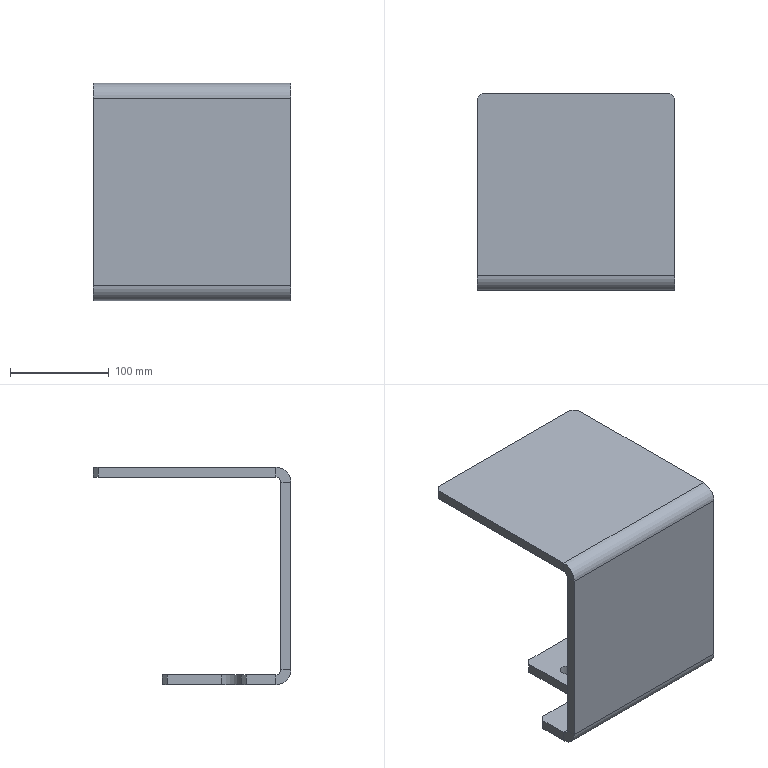Part | SolidWorks | features ICE 4, Fillet 3, Chamfer 1, Extrusion 1, FlatPattern 1, SheetMetal 1, SolidToSheetMetal 1 | 1 solid | 38 faces | box 200 x 200 x 220 mm | volume 944720 mm3 | plane 28 | cylinder 10 | commonest cylinder face diameters 14 x4 10 x2 30 x2 40 x2
STEP:
#1=CARTESIAN_POINT('',(67.,-40.,0.));
#2=VERTEX_POINT('',#1);
#3=CARTESIAN_POINT('',(53.,-40.,0.));
#4=VERTEX_POINT('',#3);
#5=CARTESIAN_POINT('',(60.,-40.,0.));
#6=DIRECTION('',(0.,0.,-1.));
#7=DIRECTION('',(1.,0.,0.));
#8=AXIS2_PLACEMENT_3D('',#5,#6,#7);
#9=CIRCLE('',#8,7.);
#10=EDGE_CURVE('',#2,#4,#9,.T.);
#11=ORIENTED_EDGE('',*,*,#10,.T.);
#12=CARTESIAN_POINT('',(53.,-40.,10.));
#13=VERTEX_POINT('',#12);
#14=CARTESIAN_POINT('',(53.,-40.,10.));
#15=DIRECTION('',(0.,0.,1.));
#16=VECTOR('',#15,1000.);
#17=LINE('',#14,#16);
#18=EDGE_CURVE('',#4,#13,#17,.T.);
#19=ORIENTED_EDGE('',*,*,#18,.T.);
#20=CARTESIAN_POINT('',(67.,-40.,10.));
#21=VERTEX_POINT('',#20);
#22=CARTESIAN_POINT('',(60.,-40.,10.));
#23=DIRECTION('',(0.,0.,-1.));
#24=DIRECTION('',(1.,0.,0.));
#25=AXIS2_PLACEMENT_3D('',#22,#23,#24);
#26=CIRCLE('',#25,7.);
#27=EDGE_CURVE('',#21,#13,#26,.T.);
#28=ORIENTED_EDGE('',*,*,#27,.F.);
#29=CARTESIAN_POINT('',(67.,-40.,10.));
#30=DIRECTION('',(0.,0.,1.));
#31=VECTOR('',#30,1000.);
#32=LINE('',#29,#31);
#33=EDGE_CURVE('',#2,#21,#32,.T.);
#34=ORIENTED_EDGE('',*,*,#33,.F.);
#35=EDGE_LOOP('',(#11,#19,#28,#34));
#36=FACE_OUTER_BOUND('',#35,.T.);
#37=CARTESIAN_POINT('',(60.,-40.,10.));
#38=DIRECTION('',(0.,0.,1.));
#39=DIRECTION('',(1.,0.,0.));
#40=AXIS2_PLACEMENT_3D('',#37,#38,#39);
#41=CYLINDRICAL_SURFACE('',#40,7.);
#42=ADVANCED_FACE('',(#36),#41,.F.);
#43=CARTESIAN_POINT('',(27.,-40.,0.));
#44=VERTEX_POINT('',#43);
#45=CARTESIAN_POINT('',(13.,-40.,0.));
#46=VERTEX_POINT('',#45);
#47=CARTESIAN_POINT('',(20.,-40.,0.));
#48=DIRECTION('',(0.,0.,-1.));
#49=DIRECTION('',(1.,0.,0.));
#50=AXIS2_PLACEMENT_3D('',#47,#48,#49);
#51=CIRCLE('',#50,7.);
#52=EDGE_CURVE('',#44,#46,#51,.T.);
#53=ORIENTED_EDGE('',*,*,#52,.T.);
#54=CARTESIAN_POINT('',(13.,-40.,10.));
#55=VERTEX_POINT('',#54);
#56=CARTESIAN_POINT('',(13.,-40.,10.));
#57=DIRECTION('',(0.,0.,1.));
#58=VECTOR('',#57,1000.);
#59=LINE('',#56,#58);
#60=EDGE_CURVE('',#46,#55,#59,.T.);
#61=ORIENTED_EDGE('',*,*,#60,.T.);
#62=CARTESIAN_POINT('',(27.,-40.,10.));
#63=VERTEX_POINT('',#62);
#64=CARTESIAN_POINT('',(20.,-40.,10.));
#65=DIRECTION('',(0.,0.,-1.));
#66=DIRECTION('',(1.,0.,0.));
#67=AXIS2_PLACEMENT_3D('',#64,#65,#66);
#68=CIRCLE('',#67,7.);
#69=EDGE_CURVE('',#63,#55,#68,.T.);
#70=ORIENTED_EDGE('',*,*,#69,.F.);
#71=CARTESIAN_POINT('',(27.,-40.,10.));
#72=DIRECTION('',(0.,0.,1.));
#73=VECTOR('',#72,1000.);
#74=LINE('',#71,#73);
#75=EDGE_CURVE('',#44,#63,#74,.T.);
#76=ORIENTED_EDGE('',*,*,#75,.F.);
#77=EDGE_LOOP('',(#53,#61,#70,#76));
#78=FACE_OUTER_BOUND('',#77,.T.);
#79=CARTESIAN_POINT('',(20.,-40.,10.));
#80=DIRECTION('',(0.,0.,1.));
#81=DIRECTION('',(1.,0.,0.));
#82=AXIS2_PLACEMENT_3D('',#79,#80,#81);
#83=CYLINDRICAL_SURFACE('',#82,7.);
#84=ADVANCED_FACE('',(#78),#83,.F.);
#85=CARTESIAN_POINT('',(140.,-130.,15.));
#86=VERTEX_POINT('',#85);
#87=CARTESIAN_POINT('',(140.,-120.,15.));
#88=VERTEX_POINT('',#87);
#89=CARTESIAN_POINT('',(140.,-120.,15.));
#90=DIRECTION('',(0.,1.,0.));
#91=VECTOR('',#90,1000.);
#92=LINE('',#89,#91);
#93=EDGE_CURVE('',#86,#88,#92,.T.);
#94=ORIENTED_EDGE('',*,*,#93,.F.);
#95=CARTESIAN_POINT('',(140.,-115.,0.));
#96=VERTEX_POINT('',#95);
#97=CARTESIAN_POINT('',(140.,-115.,15.));
#98=DIRECTION('',(-1.,0.,0.));
#99=DIRECTION('',(0.,0.,1.));
#100=AXIS2_PLACEMENT_3D('',#97,#98,#99);
#101=CIRCLE('',#100,15.);
#102=EDGE_CURVE('',#96,#86,#101,.T.);
#103=ORIENTED_EDGE('',*,*,#102,.F.);
#104=CARTESIAN_POINT('',(140.,-115.,10.));
#105=VERTEX_POINT('',#104);
#106=CARTESIAN_POINT('',(140.,-115.,10.));
#107=DIRECTION('',(0.,0.,1.));
#108=VECTOR('',#107,1000.);
#109=LINE('',#106,#108);
#110=EDGE_CURVE('',#96,#105,#109,.T.);
#111=ORIENTED_EDGE('',*,*,#110,.T.);
#112=CARTESIAN_POINT('',(140.,-115.,15.));
#113=DIRECTION('',(-1.,0.,0.));
#114=DIRECTION('',(0.,1.,0.));
#115=AXIS2_PLACEMENT_3D('',#112,#113,#114);
#116=CIRCLE('',#115,5.);
#117=EDGE_CURVE('',#105,#88,#116,.T.);
#118=ORIENTED_EDGE('',*,*,#117,.T.);
#119=EDGE_LOOP('',(#94,#103,#111,#118));
#120=FACE_OUTER_BOUND('',#119,.T.);
#121=CARTESIAN_POINT('',(140.,-115.,15.));
#122=DIRECTION('',(-1.,0.,0.));
#123=DIRECTION('',(0.,-1.,0.));
#124=AXIS2_PLACEMENT_3D('',#121,#122,#123);
#125=PLANE('',#124);
#126=ADVANCED_FACE('',(#120),#125,.F.);
#127=ORIENTED_EDGE('',*,*,#110,.F.);
#128=CARTESIAN_POINT('',(140.,-85.,0.));
#129=VERTEX_POINT('',#128);
#130=CARTESIAN_POINT('',(140.,0.,0.));
#131=DIRECTION('',(0.,1.,0.));
#132=VECTOR('',#131,1000.);
#133=LINE('',#130,#132);
#134=EDGE_CURVE('',#96,#129,#133,.T.);
#135=ORIENTED_EDGE('',*,*,#134,.T.);
#136=CARTESIAN_POINT('',(140.,-85.,10.));
#137=VERTEX_POINT('',#136);
#138=CARTESIAN_POINT('',(140.,-85.,10.));
#139=DIRECTION('',(0.,0.,1.));
#140=VECTOR('',#139,1000.);
#141=LINE('',#138,#140);
#142=EDGE_CURVE('',#129,#137,#141,.T.);
#143=ORIENTED_EDGE('',*,*,#142,.T.);
#144=CARTESIAN_POINT('',(140.,-80.,10.));
#145=DIRECTION('',(0.,1.,0.));
#146=VECTOR('',#145,1000.);
#147=LINE('',#144,#146);
#148=EDGE_CURVE('',#105,#137,#147,.T.);
#149=ORIENTED_EDGE('',*,*,#148,.F.);
#150=EDGE_LOOP('',(#127,#135,#143,#149));
#151=FACE_OUTER_BOUND('',#150,.T.);
#152=CARTESIAN_POINT('',(140.,-80.,10.));
#153=DIRECTION('',(1.,0.,0.));
#154=DIRECTION('',(0.,1.,0.));
#155=AXIS2_PLACEMENT_3D('',#152,#153,#154);
#156=PLANE('',#155);
#157=ADVANCED_FACE('',(#151),#156,.T.);
#158=ORIENTED_EDGE('',*,*,#142,.F.);
#159=CARTESIAN_POINT('',(135.,-80.,0.));
#160=VERTEX_POINT('',#159);
#161=CARTESIAN_POINT('',(27.5,27.5,0.));
#162=DIRECTION('',(-0.7071,0.7071,0.));
#163=VECTOR('',#162,1000.);
#164=LINE('',#161,#163);
#165=EDGE_CURVE('',#129,#160,#164,.T.);
#166=ORIENTED_EDGE('',*,*,#165,.T.);
#167=CARTESIAN_POINT('',(135.,-80.,10.));
#168=VERTEX_POINT('',#167);
#169=CARTESIAN_POINT('',(135.,-80.,10.));
#170=DIRECTION('',(0.,0.,1.));
#171=VECTOR('',#170,1000.);
#172=LINE('',#169,#171);
#173=EDGE_CURVE('',#160,#168,#172,.T.);
#174=ORIENTED_EDGE('',*,*,#173,.T.);
#175=CARTESIAN_POINT('',(27.5,27.5,10.));
#176=DIRECTION('',(-0.7071,0.7071,0.));
#177=VECTOR('',#176,1000.);
#178=LINE('',#175,#177);
#179=EDGE_CURVE('',#137,#168,#178,.T.);
#180=ORIENTED_EDGE('',*,*,#179,.F.);
#181=EDGE_LOOP('',(#158,#166,#174,#180));
#182=FACE_OUTER_BOUND('',#181,.T.);
#183=CARTESIAN_POINT('',(27.5,27.5,10.));
#184=DIRECTION('',(-0.7071,-0.7071,0.));
#185=DIRECTION('',(0.7071,-0.7071,0.));
#186=AXIS2_PLACEMENT_3D('',#183,#184,#185);
#187=PLANE('',#186);
#188=ADVANCED_FACE('',(#182),#187,.F.);
#189=ORIENTED_EDGE('',*,*,#173,.F.);
#190=CARTESIAN_POINT('',(100.,-80.,0.));
#191=VERTEX_POINT('',#190);
#192=CARTESIAN_POINT('',(0.,-80.,0.));
#193=DIRECTION('',(-1.,0.,0.));
#194=VECTOR('',#193,1000.);
#195=LINE('',#192,#194);
#196=EDGE_CURVE('',#160,#191,#195,.T.);
#197=ORIENTED_EDGE('',*,*,#196,.T.);
#198=CARTESIAN_POINT('',(100.,-80.,10.));
#199=VERTEX_POINT('',#198);
#200=CARTESIAN_POINT('',(100.,-80.,10.));
#201=DIRECTION('',(0.,0.,1.));
#202=VECTOR('',#201,1000.);
#203=LINE('',#200,#202);
#204=EDGE_CURVE('',#191,#199,#203,.T.);
#205=ORIENTED_EDGE('',*,*,#204,.T.);
#206=CARTESIAN_POINT('',(-60.,-80.,10.));
#207=DIRECTION('',(-1.,0.,0.));
#208=VECTOR('',#207,1000.);
#209=LINE('',#206,#208);
#210=EDGE_CURVE('',#168,#199,#209,.T.);
#211=ORIENTED_EDGE('',*,*,#210,.F.);
#212=EDGE_LOOP('',(#189,#197,#205,#211));
#213=FACE_OUTER_BOUND('',#212,.T.);
#214=CARTESIAN_POINT('',(-60.,-80.,10.));
#215=DIRECTION('',(0.,1.,0.));
#216=DIRECTION('',(-1.,0.,0.));
#217=AXIS2_PLACEMENT_3D('',#214,#215,#216);
#218=PLANE('',#217);
#219=ADVANCED_FACE('',(#213),#218,.T.);
#220=ORIENTED_EDGE('',*,*,#204,.F.);
#221=CARTESIAN_POINT('',(80.,-60.,0.));
#222=VERTEX_POINT('',#221);
#223=CARTESIAN_POINT('',(100.,-60.,0.));
#224=DIRECTION('',(0.,0.,-1.));
#225=DIRECTION('',(1.,0.,0.));
#226=AXIS2_PLACEMENT_3D('',#223,#224,#225);
#227=CIRCLE('',#226,20.);
#228=EDGE_CURVE('',#191,#222,#227,.T.);
#229=ORIENTED_EDGE('',*,*,#228,.T.);
#230=CARTESIAN_POINT('',(80.,-60.,10.));
#231=VERTEX_POINT('',#230);
#232=CARTESIAN_POINT('',(80.,-60.,10.));
#233=DIRECTION('',(0.,0.,1.));
#234=VECTOR('',#233,1000.);
#235=LINE('',#232,#234);
#236=EDGE_CURVE('',#222,#231,#235,.T.);
#237=ORIENTED_EDGE('',*,*,#236,.T.);
#238=CARTESIAN_POINT('',(100.,-60.,10.));
#239=DIRECTION('',(0.,0.,-1.));
#240=DIRECTION('',(1.,0.,0.));
#241=AXIS2_PLACEMENT_3D('',#238,#239,#240);
#242=CIRCLE('',#241,20.);
#243=EDGE_CURVE('',#199,#231,#242,.T.);
#244=ORIENTED_EDGE('',*,*,#243,.F.);
#245=EDGE_LOOP('',(#220,#229,#237,#244));
#246=FACE_OUTER_BOUND('',#245,.T.);
#247=CARTESIAN_POINT('',(100.,-60.,10.));
#248=DIRECTION('',(0.,0.,1.));
#249=DIRECTION('',(1.,0.,0.));
#250=AXIS2_PLACEMENT_3D('',#247,#248,#249);
#251=CYLINDRICAL_SURFACE('',#250,20.);
#252=ADVANCED_FACE('',(#246),#251,.F.);
#253=ORIENTED_EDGE('',*,*,#236,.F.);
#254=CARTESIAN_POINT('',(80.,-5.,0.));
#255=VERTEX_POINT('',#254);
#256=CARTESIAN_POINT('',(80.,0.,0.));
#257=DIRECTION('',(0.,1.,0.));
#258=VECTOR('',#257,1000.);
#259=LINE('',#256,#258);
#260=EDGE_CURVE('',#222,#255,#259,.T.);
#261=ORIENTED_EDGE('',*,*,#260,.T.);
#262=CARTESIAN_POINT('',(80.,-5.,10.));
#263=VERTEX_POINT('',#262);
#264=CARTESIAN_POINT('',(80.,-5.,10.));
#265=DIRECTION('',(0.,0.,1.));
#266=VECTOR('',#265,1000.);
#267=LINE('',#264,#266);
#268=EDGE_CURVE('',#255,#263,#267,.T.);
#269=ORIENTED_EDGE('',*,*,#268,.T.);
#270=CARTESIAN_POINT('',(80.,0.,10.));
#271=DIRECTION('',(0.,1.,0.));
#272=VECTOR('',#271,1000.);
#273=LINE('',#270,#272);
#274=EDGE_CURVE('',#231,#263,#273,.T.);
#275=ORIENTED_EDGE('',*,*,#274,.F.);
#276=EDGE_LOOP('',(#253,#261,#269,#275));
#277=FACE_OUTER_BOUND('',#276,.T.);
#278=CARTESIAN_POINT('',(80.,0.,10.));
#279=DIRECTION('',(1.,0.,0.));
#280=DIRECTION('',(0.,1.,0.));
#281=AXIS2_PLACEMENT_3D('',#278,#279,#280);
#282=PLANE('',#281);
#283=ADVANCED_FACE('',(#277),#282,.T.);
#284=ORIENTED_EDGE('',*,*,#268,.F.);
#285=CARTESIAN_POINT('',(75.,0.,0.));
#286=VERTEX_POINT('',#285);
#287=CARTESIAN_POINT('',(37.5,37.5,0.));
#288=DIRECTION('',(-0.7071,0.7071,0.));
#289=VECTOR('',#288,1000.);
#290=LINE('',#287,#289);
#291=EDGE_CURVE('',#255,#286,#290,.T.);
#292=ORIENTED_EDGE('',*,*,#291,.T.);
#293=CARTESIAN_POINT('',(75.,0.,10.));
#294=VERTEX_POINT('',#293);
#295=CARTESIAN_POINT('',(75.,0.,10.));
#296=DIRECTION('',(0.,0.,1.));
#297=VECTOR('',#296,1000.);
#298=LINE('',#295,#297);
#299=EDGE_CURVE('',#286,#294,#298,.T.);
#300=ORIENTED_EDGE('',*,*,#299,.T.);
#301=CARTESIAN_POINT('',(37.5,37.5,10.));
#302=DIRECTION('',(-0.7071,0.7071,0.));
#303=VECTOR('',#302,1000.);
#304=LINE('',#301,#303);
#305=EDGE_CURVE('',#263,#294,#304,.T.);
#306=ORIENTED_EDGE('',*,*,#305,.F.);
#307=EDGE_LOOP('',(#284,#292,#300,#306));
#308=FACE_OUTER_BOUND('',#307,.T.);
#309=CARTESIAN_POINT('',(37.5,37.5,10.));
#310=DIRECTION('',(-0.7071,-0.7071,0.));
#311=DIRECTION('',(0.7071,-0.7071,0.));
#312=AXIS2_PLACEMENT_3D('',#309,#310,#311);
#313=PLANE('',#312);
#314=ADVANCED_FACE('',(#308),#313,.F.);
#315=ORIENTED_EDGE('',*,*,#299,.F.);
#316=CARTESIAN_POINT('',(5.,0.,0.));
#317=VERTEX_POINT('',#316);
#318=CARTESIAN_POINT('',(0.,0.,0.));
#319=DIRECTION('',(-1.,0.,0.));
#320=VECTOR('',#319,1000.);
#321=LINE('',#318,#320);
#322=EDGE_CURVE('',#286,#317,#321,.T.);
#323=ORIENTED_EDGE('',*,*,#322,.T.);
#324=CARTESIAN_POINT('',(5.,0.,10.));
#325=VERTEX_POINT('',#324);
#326=CARTESIAN_POINT('',(5.,0.,10.));
#327=DIRECTION('',(0.,0.,1.));
#328=VECTOR('',#327,1000.);
#329=LINE('',#326,#328);
#330=EDGE_CURVE('',#317,#325,#329,.T.);
#331=ORIENTED_EDGE('',*,*,#330,.T.);
#332=CARTESIAN_POINT('',(0.,0.,10.));
#333=DIRECTION('',(-1.,0.,0.));
#334=VECTOR('',#333,1000.);
#335=LINE('',#332,#334);
#336=EDGE_CURVE('',#294,#325,#335,.T.);
#337=ORIENTED_EDGE('',*,*,#336,.F.);
#338=EDGE_LOOP('',(#315,#323,#331,#337));
#339=FACE_OUTER_BOUND('',#338,.T.);
#340=CARTESIAN_POINT('',(0.,0.,10.));
#341=DIRECTION('',(0.,1.,0.));
#342=DIRECTION('',(-1.,0.,0.));
#343=AXIS2_PLACEMENT_3D('',#340,#341,#342);
#344=PLANE('',#343);
#345=ADVANCED_FACE('',(#339),#344,.T.);
#346=ORIENTED_EDGE('',*,*,#330,.F.);
#347=CARTESIAN_POINT('',(0.,-5.,0.));
#348=VERTEX_POINT('',#347);
#349=CARTESIAN_POINT('',(2.5,-2.5,0.));
#350=DIRECTION('',(-0.7071,-0.7071,0.));
#351=VECTOR('',#350,1000.);
#352=LINE('',#349,#351);
#353=EDGE_CURVE('',#317,#348,#352,.T.);
#354=ORIENTED_EDGE('',*,*,#353,.T.);
#355=CARTESIAN_POINT('',(0.,-5.,10.));
#356=VERTEX_POINT('',#355);
#357=CARTESIAN_POINT('',(0.,-5.,10.));
#358=DIRECTION('',(0.,0.,1.));
#359=VECTOR('',#358,1000.);
#360=LINE('',#357,#359);
#361=EDGE_CURVE('',#348,#356,#360,.T.);
#362=ORIENTED_EDGE('',*,*,#361,.T.);
#363=CARTESIAN_POINT('',(2.5,-2.5,10.));
#364=DIRECTION('',(-0.7071,-0.7071,0.));
#365=VECTOR('',#364,1000.);
#366=LINE('',#363,#365);
#367=EDGE_CURVE('',#325,#356,#366,.T.);
#368=ORIENTED_EDGE('',*,*,#367,.F.);
#369=EDGE_LOOP('',(#346,#354,#362,#368));
#370=FACE_OUTER_BOUND('',#369,.T.);
#371=CARTESIAN_POINT('',(2.5,-2.5,10.));
#372=DIRECTION('',(0.7071,-0.7071,0.));
#373=DIRECTION('',(0.7071,0.7071,0.));
#374=AXIS2_PLACEMENT_3D('',#371,#372,#373);
#375=PLANE('',#374);
#376=ADVANCED_FACE('',(#370),#375,.F.);
#377=ORIENTED_EDGE('',*,*,#361,.F.);
#378=CARTESIAN_POINT('',(0.,-60.,0.));
#379=VERTEX_POINT('',#378);
#380=CARTESIAN_POINT('',(0.,0.,0.));
#381=DIRECTION('',(0.,-1.,0.));
#382=VECTOR('',#381,1000.);
#383=LINE('',#380,#382);
#384=EDGE_CURVE('',#348,#379,#383,.T.);
#385=ORIENTED_EDGE('',*,*,#384,.T.);
#386=CARTESIAN_POINT('',(0.,-60.,10.));
#387=VERTEX_POINT('',#386);
#388=CARTESIAN_POINT('',(0.,-60.,10.));
#389=DIRECTION('',(0.,0.,1.));
#390=VECTOR('',#389,1000.);
#391=LINE('',#388,#390);
#392=EDGE_CURVE('',#379,#387,#391,.T.);
#393=ORIENTED_EDGE('',*,*,#392,.T.);
#394=CARTESIAN_POINT('',(0.,0.,10.));
#395=DIRECTION('',(0.,-1.,0.));
#396=VECTOR('',#395,1000.);
#397=LINE('',#394,#396);
#398=EDGE_CURVE('',#356,#387,#397,.T.);
#399=ORIENTED_EDGE('',*,*,#398,.F.);
#400=EDGE_LOOP('',(#377,#385,#393,#399));
#401=FACE_OUTER_BOUND('',#400,.T.);
#402=CARTESIAN_POINT('',(0.,0.,10.));
#403=DIRECTION('',(-1.,0.,0.));
#404=DIRECTION('',(0.,-1.,0.));
#405=AXIS2_PLACEMENT_3D('',#402,#403,#404);
#406=PLANE('',#405);
#407=ADVANCED_FACE('',(#401),#406,.T.);
#408=ORIENTED_EDGE('',*,*,#392,.F.);
#409=CARTESIAN_POINT('',(-20.,-80.,0.));
#410=VERTEX_POINT('',#409);
#411=CARTESIAN_POINT('',(-20.,-60.,0.));
#412=DIRECTION('',(0.,0.,-1.));
#413=DIRECTION('',(1.,0.,0.));
#414=AXIS2_PLACEMENT_3D('',#411,#412,#413);
#415=CIRCLE('',#414,20.);
#416=EDGE_CURVE('',#379,#410,#415,.T.);
#417=ORIENTED_EDGE('',*,*,#416,.T.);
#418=CARTESIAN_POINT('',(-20.,-80.,10.));
#419=VERTEX_POINT('',#418);
#420=CARTESIAN_POINT('',(-20.,-80.,10.));
#421=DIRECTION('',(0.,0.,1.));
#422=VECTOR('',#421,1000.);
#423=LINE('',#420,#422);
#424=EDGE_CURVE('',#410,#419,#423,.T.);
#425=ORIENTED_EDGE('',*,*,#424,.T.);
#426=CARTESIAN_POINT('',(-20.,-60.,10.));
#427=DIRECTION('',(0.,0.,-1.));
#428=DIRECTION('',(1.,0.,0.));
#429=AXIS2_PLACEMENT_3D('',#426,#427,#428);
#430=CIRCLE('',#429,20.);
#431=EDGE_CURVE('',#387,#419,#430,.T.);
#432=ORIENTED_EDGE('',*,*,#431,.F.);
#433=EDGE_LOOP('',(#408,#417,#425,#432));
#434=FACE_OUTER_BOUND('',#433,.T.);
#435=CARTESIAN_POINT('',(-20.,-60.,10.));
#436=DIRECTION('',(0.,0.,1.));
#437=DIRECTION('',(1.,0.,0.));
#438=AXIS2_PLACEMENT_3D('',#435,#436,#437);
#439=CYLINDRICAL_SURFACE('',#438,20.);
#440=ADVANCED_FACE('',(#434),#439,.F.);
#441=ORIENTED_EDGE('',*,*,#424,.F.);
#442=CARTESIAN_POINT('',(-55.,-80.,0.));
#443=VERTEX_POINT('',#442);
#444=CARTESIAN_POINT('',(0.,-80.,0.));
#445=DIRECTION('',(-1.,0.,0.));
#446=VECTOR('',#445,1000.);
#447=LINE('',#444,#446);
#448=EDGE_CURVE('',#410,#443,#447,.T.);
#449=ORIENTED_EDGE('',*,*,#448,.T.);
#450=CARTESIAN_POINT('',(-55.,-80.,10.));
#451=VERTEX_POINT('',#450);
#452=CARTESIAN_POINT('',(-55.,-80.,10.));
#453=DIRECTION('',(0.,0.,1.));
#454=VECTOR('',#453,1000.);
#455=LINE('',#452,#454);
#456=EDGE_CURVE('',#443,#451,#455,.T.);
#457=ORIENTED_EDGE('',*,*,#456,.T.);
#458=CARTESIAN_POINT('',(-60.,-80.,10.));
#459=DIRECTION('',(-1.,0.,0.));
#460=VECTOR('',#459,1000.);
#461=LINE('',#458,#460);
#462=EDGE_CURVE('',#419,#451,#461,.T.);
#463=ORIENTED_EDGE('',*,*,#462,.F.);
#464=EDGE_LOOP('',(#441,#449,#457,#463));
#465=FACE_OUTER_BOUND('',#464,.T.);
#466=CARTESIAN_POINT('',(-60.,-80.,10.));
#467=DIRECTION('',(0.,1.,0.));
#468=DIRECTION('',(-1.,0.,0.));
#469=AXIS2_PLACEMENT_3D('',#466,#467,#468);
#470=PLANE('',#469);
#471=ADVANCED_FACE('',(#465),#470,.T.);
#472=ORIENTED_EDGE('',*,*,#456,.F.);
#473=CARTESIAN_POINT('',(-60.,-85.,0.));
#474=VERTEX_POINT('',#473);
#475=CARTESIAN_POINT('',(12.5,-12.5,0.));
#476=DIRECTION('',(-0.7071,-0.7071,0.));
#477=VECTOR('',#476,1000.);
#478=LINE('',#475,#477);
#479=EDGE_CURVE('',#443,#474,#478,.T.);
#480=ORIENTED_EDGE('',*,*,#479,.T.);
#481=CARTESIAN_POINT('',(-60.,-85.,10.));
#482=VERTEX_POINT('',#481);
#483=CARTESIAN_POINT('',(-60.,-85.,10.));
#484=DIRECTION('',(0.,0.,1.));
#485=VECTOR('',#484,1000.);
#486=LINE('',#483,#485);
#487=EDGE_CURVE('',#474,#482,#486,.T.);
#488=ORIENTED_EDGE('',*,*,#487,.T.);
#489=CARTESIAN_POINT('',(12.5,-12.5,10.));
#490=DIRECTION('',(-0.7071,-0.7071,0.));
#491=VECTOR('',#490,1000.);
#492=LINE('',#489,#491);
#493=EDGE_CURVE('',#451,#482,#492,.T.);
#494=ORIENTED_EDGE('',*,*,#493,.F.);
#495=EDGE_LOOP('',(#472,#480,#488,#494));
#496=FACE_OUTER_BOUND('',#495,.T.);
#497=CARTESIAN_POINT('',(12.5,-12.5,10.));
#498=DIRECTION('',(0.7071,-0.7071,0.));
#499=DIRECTION('',(0.7071,0.7071,0.));
#500=AXIS2_PLACEMENT_3D('',#497,#498,#499);
#501=PLANE('',#500);
#502=ADVANCED_FACE('',(#496),#501,.F.);
#503=ORIENTED_EDGE('',*,*,#487,.F.);
#504=CARTESIAN_POINT('',(-60.,-115.,0.));
#505=VERTEX_POINT('',#504);
#506=CARTESIAN_POINT('',(-60.,0.,0.));
#507=DIRECTION('',(0.,-1.,0.));
#508=VECTOR('',#507,1000.);
#509=LINE('',#506,#508);
#510=EDGE_CURVE('',#474,#505,#509,.T.);
#511=ORIENTED_EDGE('',*,*,#510,.T.);
#512=CARTESIAN_POINT('',(-60.,-115.,10.));
#513=VERTEX_POINT('',#512);
#514=CARTESIAN_POINT('',(-60.,-115.,10.));
#515=DIRECTION('',(0.,0.,1.));
#516=VECTOR('',#515,1000.);
#517=LINE('',#514,#516);
#518=EDGE_CURVE('',#505,#513,#517,.T.);
#519=ORIENTED_EDGE('',*,*,#518,.T.);
#520=CARTESIAN_POINT('',(-60.,-80.,10.));
#521=DIRECTION('',(0.,-1.,0.));
#522=VECTOR('',#521,1000.);
#523=LINE('',#520,#522);
#524=EDGE_CURVE('',#482,#513,#523,.T.);
#525=ORIENTED_EDGE('',*,*,#524,.F.);
#526=EDGE_LOOP('',(#503,#511,#519,#525));
#527=FACE_OUTER_BOUND('',#526,.T.);
#528=CARTESIAN_POINT('',(-60.,-80.,10.));
#529=DIRECTION('',(-1.,0.,0.));
#530=DIRECTION('',(0.,-1.,0.));
#531=AXIS2_PLACEMENT_3D('',#528,#529,#530);
#532=PLANE('',#531);
#533=ADVANCED_FACE('',(#527),#532,.T.);
#534=ORIENTED_EDGE('',*,*,#518,.F.);
#535=CARTESIAN_POINT('',(-60.,-130.,15.));
#536=VERTEX_POINT('',#535);
#537=CARTESIAN_POINT('',(-60.,-115.,15.));
#538=DIRECTION('',(1.,0.,0.));
#539=DIRECTION('',(0.,0.,1.));
#540=AXIS2_PLACEMENT_3D('',#537,#538,#539);
#541=CIRCLE('',#540,15.);
#542=EDGE_CURVE('',#536,#505,#541,.T.);
#543=ORIENTED_EDGE('',*,*,#542,.F.);
#544=CARTESIAN_POINT('',(-60.,-120.,15.));
#545=VERTEX_POINT('',#544);
#546=CARTESIAN_POINT('',(-60.,-120.,15.));
#547=DIRECTION('',(0.,1.,0.));
#548=VECTOR('',#547,1000.);
#549=LINE('',#546,#548);
#550=EDGE_CURVE('',#536,#545,#549,.T.);
#551=ORIENTED_EDGE('',*,*,#550,.T.);
#552=CARTESIAN_POINT('',(-60.,-115.,15.));
#553=DIRECTION('',(1.,0.,0.));
#554=DIRECTION('',(0.,-1.,0.));
#555=AXIS2_PLACEMENT_3D('',#552,#553,#554);
#556=CIRCLE('',#555,5.);
#557=EDGE_CURVE('',#545,#513,#556,.T.);
#558=ORIENTED_EDGE('',*,*,#557,.T.);
#559=EDGE_LOOP('',(#534,#543,#551,#558));
#560=FACE_OUTER_BOUND('',#559,.T.);
#561=CARTESIAN_POINT('',(-60.,-115.,15.));
#562=DIRECTION('',(1.,0.,0.));
#563=DIRECTION('',(0.,1.,0.));
#564=AXIS2_PLACEMENT_3D('',#561,#562,#563);
#565=PLANE('',#564);
#566=ADVANCED_FACE('',(#560),#565,.F.);
#567=ORIENTED_EDGE('',*,*,#550,.F.);
#568=CARTESIAN_POINT('',(-60.,-130.,205.));
#569=VERTEX_POINT('',#568);
#570=CARTESIAN_POINT('',(-60.,-130.,210.));
#571=DIRECTION('',(0.,0.,-1.));
#572=VECTOR('',#571,1000.);
#573=LINE('',#570,#572);
#574=EDGE_CURVE('',#569,#536,#573,.T.);
#575=ORIENTED_EDGE('',*,*,#574,.F.);
#576=CARTESIAN_POINT('',(-60.,-120.,205.));
#577=VERTEX_POINT('',#576);
#578=CARTESIAN_POINT('',(-60.,-120.,205.));
#579=DIRECTION('',(0.,1.,0.));
#580=VECTOR('',#579,1000.);
#581=LINE('',#578,#580);
#582=EDGE_CURVE('',#569,#577,#581,.T.);
#583=ORIENTED_EDGE('',*,*,#582,.T.);
#584=CARTESIAN_POINT('',(-60.,-120.,210.));
#585=DIRECTION('',(0.,0.,-1.));
#586=VECTOR('',#585,1000.);
#587=LINE('',#584,#586);
#588=EDGE_CURVE('',#577,#545,#587,.T.);
#589=ORIENTED_EDGE('',*,*,#588,.T.);
#590=EDGE_LOOP('',(#567,#575,#583,#589));
#591=FACE_OUTER_BOUND('',#590,.T.);
#592=CARTESIAN_POINT('',(-60.,-120.,210.));
#593=DIRECTION('',(-1.,0.,0.));
#594=DIRECTION('',(0.,0.,-1.));
#595=AXIS2_PLACEMENT_3D('',#592,#593,#594);
#596=PLANE('',#595);
#597=ADVANCED_FACE('',(#591),#596,.T.);
#598=ORIENTED_EDGE('',*,*,#582,.F.);
#599=CARTESIAN_POINT('',(-60.,-115.,220.));
#600=VERTEX_POINT('',#599);
#601=CARTESIAN_POINT('',(-60.,-115.,205.));
#602=DIRECTION('',(1.,0.,0.));
#603=DIRECTION('',(0.,0.,1.));
#604=AXIS2_PLACEMENT_3D('',#601,#602,#603);
#605=CIRCLE('',#604,15.);
#606=EDGE_CURVE('',#600,#569,#605,.T.);
#607=ORIENTED_EDGE('',*,*,#606,.F.);
#608=CARTESIAN_POINT('',(-60.,-115.,210.));
#609=VERTEX_POINT('',#608);
#610=CARTESIAN_POINT('',(-60.,-115.,210.));
#611=DIRECTION('',(0.,0.,-1.));
#612=VECTOR('',#611,1000.);
#613=LINE('',#610,#612);
#614=EDGE_CURVE('',#600,#609,#613,.T.);
#615=ORIENTED_EDGE('',*,*,#614,.T.);
#616=CARTESIAN_POINT('',(-60.,-115.,205.));
#617=DIRECTION('',(1.,0.,0.));
#618=DIRECTION('',(0.,-1.,0.));
#619=AXIS2_PLACEMENT_3D('',#616,#617,#618);
#620=CIRCLE('',#619,5.);
#621=EDGE_CURVE('',#609,#577,#620,.T.);
#622=ORIENTED_EDGE('',*,*,#621,.T.);
#623=EDGE_LOOP('',(#598,#607,#615,#622));
#624=FACE_OUTER_BOUND('',#623,.T.);
#625=CARTESIAN_POINT('',(-60.,-115.,205.));
#626=DIRECTION('',(1.,0.,0.));
#627=DIRECTION('',(0.,1.,0.));
#628=AXIS2_PLACEMENT_3D('',#625,#626,#627);
#629=PLANE('',#628);
#630=ADVANCED_FACE('',(#624),#629,.F.);
#631=ORIENTED_EDGE('',*,*,#614,.F.);
#632=CARTESIAN_POINT('',(-60.,65.,220.));
#633=VERTEX_POINT('',#632);
#634=CARTESIAN_POINT('',(-60.,0.,220.));
#635=DIRECTION('',(0.,-1.,0.));
#636=VECTOR('',#635,1000.);
#637=LINE('',#634,#636);
#638=EDGE_CURVE('',#633,#600,#637,.T.);
#639=ORIENTED_EDGE('',*,*,#638,.F.);
#640=CARTESIAN_POINT('',(-60.,65.,210.));
#641=VERTEX_POINT('',#640);
#642=CARTESIAN_POINT('',(-60.,65.,210.));
#643=DIRECTION('',(0.,0.,-1.));
#644=VECTOR('',#643,1000.);
#645=LINE('',#642,#644);
#646=EDGE_CURVE('',#633,#641,#645,.T.);
#647=ORIENTED_EDGE('',*,*,#646,.T.);
#648=CARTESIAN_POINT('',(-60.,-130.,210.));
#649=DIRECTION('',(0.,-1.,0.));
#650=VECTOR('',#649,1000.);
#651=LINE('',#648,#650);
#652=EDGE_CURVE('',#641,#609,#651,.T.);
#653=ORIENTED_EDGE('',*,*,#652,.T.);
#654=EDGE_LOOP('',(#631,#639,#647,#653));
#655=FACE_OUTER_BOUND('',#654,.T.);
#656=CARTESIAN_POINT('',(-60.,-130.,210.));
#657=DIRECTION('',(1.,0.,0.));
#658=DIRECTION('',(0.,-1.,0.));
#659=AXIS2_PLACEMENT_3D('',#656,#657,#658);
#660=PLANE('',#659);
#661=ADVANCED_FACE('',(#655),#660,.F.);
#662=ORIENTED_EDGE('',*,*,#646,.F.);
#663=CARTESIAN_POINT('',(-55.,70.,220.));
#664=VERTEX_POINT('',#663);
#665=CARTESIAN_POINT('',(-62.5,62.5,220.));
#666=DIRECTION('',(0.7071,0.7071,0.));
#667=VECTOR('',#666,1000.);
#668=LINE('',#665,#667);
#669=EDGE_CURVE('',#633,#664,#668,.T.);
#670=ORIENTED_EDGE('',*,*,#669,.T.);
#671=CARTESIAN_POINT('',(-55.,70.,210.));
#672=VERTEX_POINT('',#671);
#673=CARTESIAN_POINT('',(-55.,70.,210.));
#674=DIRECTION('',(0.,0.,-1.));
#675=VECTOR('',#674,1000.);
#676=LINE('',#673,#675);
#677=EDGE_CURVE('',#664,#672,#676,.T.);
#678=ORIENTED_EDGE('',*,*,#677,.T.);
#679=CARTESIAN_POINT('',(-62.5,62.5,210.));
#680=DIRECTION('',(0.7071,0.7071,0.));
#681=VECTOR('',#680,1000.);
#682=LINE('',#679,#681);
#683=EDGE_CURVE('',#641,#672,#682,.T.);
#684=ORIENTED_EDGE('',*,*,#683,.F.);
#685=EDGE_LOOP('',(#662,#670,#678,#684));
#686=FACE_OUTER_BOUND('',#685,.T.);
#687=CARTESIAN_POINT('',(-62.5,62.5,210.));
#688=DIRECTION('',(-0.7071,0.7071,0.));
#689=DIRECTION('',(0.7071,0.7071,0.));
#690=AXIS2_PLACEMENT_3D('',#687,#688,#689);
#691=PLANE('',#690);
#692=ADVANCED_FACE('',(#686),#691,.T.);
#693=ORIENTED_EDGE('',*,*,#677,.F.);
#694=CARTESIAN_POINT('',(135.,70.,220.));
#695=VERTEX_POINT('',#694);
#696=CARTESIAN_POINT('',(0.,70.,220.));
#697=DIRECTION('',(-1.,0.,0.));
#698=VECTOR('',#697,1000.);
#699=LINE('',#696,#698);
#700=EDGE_CURVE('',#695,#664,#699,.T.);
#701=ORIENTED_EDGE('',*,*,#700,.F.);
#702=CARTESIAN_POINT('',(135.,70.,210.));
#703=VERTEX_POINT('',#702);
#704=CARTESIAN_POINT('',(135.,70.,210.));
#705=DIRECTION('',(0.,0.,-1.));
#706=VECTOR('',#705,1000.);
#707=LINE('',#704,#706);
#708=EDGE_CURVE('',#695,#703,#707,.T.);
#709=ORIENTED_EDGE('',*,*,#708,.T.);
#710=CARTESIAN_POINT('',(-60.,70.,210.));
#711=DIRECTION('',(-1.,0.,0.));
#712=VECTOR('',#711,1000.);
#713=LINE('',#710,#712);
#714=EDGE_CURVE('',#703,#672,#713,.T.);
#715=ORIENTED_EDGE('',*,*,#714,.T.);
#716=EDGE_LOOP('',(#693,#701,#709,#715));
#717=FACE_OUTER_BOUND('',#716,.T.);
#718=CARTESIAN_POINT('',(-60.,70.,210.));
#719=DIRECTION('',(0.,-1.,0.));
#720=DIRECTION('',(-1.,0.,0.));
#721=AXIS2_PLACEMENT_3D('',#718,#719,#720);
#722=PLANE('',#721);
#723=ADVANCED_FACE('',(#717),#722,.F.);
#724=ORIENTED_EDGE('',*,*,#708,.F.);
#725=CARTESIAN_POINT('',(140.,65.,220.));
#726=VERTEX_POINT('',#725);
#727=CARTESIAN_POINT('',(102.5,102.5,220.));
#728=DIRECTION('',(0.7071,-0.7071,0.));
#729=VECTOR('',#728,1000.);
#730=LINE('',#727,#729);
#731=EDGE_CURVE('',#695,#726,#730,.T.);
#732=ORIENTED_EDGE('',*,*,#731,.T.);
#733=CARTESIAN_POINT('',(140.,65.,210.));
#734=VERTEX_POINT('',#733);
#735=CARTESIAN_POINT('',(140.,65.,210.));
#736=DIRECTION('',(0.,0.,-1.));
#737=VECTOR('',#736,1000.);
#738=LINE('',#735,#737);
#739=EDGE_CURVE('',#726,#734,#738,.T.);
#740=ORIENTED_EDGE('',*,*,#739,.T.);
#741=CARTESIAN_POINT('',(102.5,102.5,210.));
#742=DIRECTION('',(0.7071,-0.7071,0.));
#743=VECTOR('',#742,1000.);
#744=LINE('',#741,#743);
#745=EDGE_CURVE('',#703,#734,#744,.T.);
#746=ORIENTED_EDGE('',*,*,#745,.F.);
#747=EDGE_LOOP('',(#724,#732,#740,#746));
#748=FACE_OUTER_BOUND('',#747,.T.);
#749=CARTESIAN_POINT('',(102.5,102.5,210.));
#750=DIRECTION('',(0.7071,0.7071,0.));
#751=DIRECTION('',(0.7071,-0.7071,0.));
#752=AXIS2_PLACEMENT_3D('',#749,#750,#751);
#753=PLANE('',#752);
#754=ADVANCED_FACE('',(#748),#753,.T.);
#755=ORIENTED_EDGE('',*,*,#739,.F.);
#756=CARTESIAN_POINT('',(140.,-115.,220.));
#757=VERTEX_POINT('',#756);
#758=CARTESIAN_POINT('',(140.,0.,220.));
#759=DIRECTION('',(0.,1.,0.));
#760=VECTOR('',#759,1000.);
#761=LINE('',#758,#760);
#762=EDGE_CURVE('',#757,#726,#761,.T.);
#763=ORIENTED_EDGE('',*,*,#762,.F.);
#764=CARTESIAN_POINT('',(140.,-115.,210.));
#765=VERTEX_POINT('',#764);
#766=CARTESIAN_POINT('',(140.,-115.,210.));
#767=DIRECTION('',(0.,0.,-1.));
#768=VECTOR('',#767,1000.);
#769=LINE('',#766,#768);
#770=EDGE_CURVE('',#757,#765,#769,.T.);
#771=ORIENTED_EDGE('',*,*,#770,.T.);
#772=CARTESIAN_POINT('',(140.,-130.,210.));
#773=DIRECTION('',(0.,1.,0.));
#774=VECTOR('',#773,1000.);
#775=LINE('',#772,#774);
#776=EDGE_CURVE('',#765,#734,#775,.T.);
#777=ORIENTED_EDGE('',*,*,#776,.T.);
#778=EDGE_LOOP('',(#755,#763,#771,#777));
#779=FACE_OUTER_BOUND('',#778,.T.);
#780=CARTESIAN_POINT('',(140.,-130.,210.));
#781=DIRECTION('',(-1.,0.,0.));
#782=DIRECTION('',(0.,1.,0.));
#783=AXIS2_PLACEMENT_3D('',#780,#781,#782);
#784=PLANE('',#783);
#785=ADVANCED_FACE('',(#779),#784,.F.);
#786=ORIENTED_EDGE('',*,*,#770,.F.);
#787=CARTESIAN_POINT('',(140.,-130.,205.));
#788=VERTEX_POINT('',#787);
#789=CARTESIAN_POINT('',(140.,-115.,205.));
#790=DIRECTION('',(-1.,0.,0.));
#791=DIRECTION('',(0.,0.,1.));
#792=AXIS2_PLACEMENT_3D('',#789,#790,#791);
#793=CIRCLE('',#792,15.);
#794=EDGE_CURVE('',#788,#757,#793,.T.);
#795=ORIENTED_EDGE('',*,*,#794,.F.);
#796=CARTESIAN_POINT('',(140.,-120.,205.));
#797=VERTEX_POINT('',#796);
#798=CARTESIAN_POINT('',(140.,-120.,205.));
#799=DIRECTION('',(0.,1.,0.));
#800=VECTOR('',#799,1000.);
#801=LINE('',#798,#800);
#802=EDGE_CURVE('',#788,#797,#801,.T.);
#803=ORIENTED_EDGE('',*,*,#802,.T.);
#804=CARTESIAN_POINT('',(140.,-115.,205.));
#805=DIRECTION('',(-1.,0.,0.));
#806=DIRECTION('',(0.,1.,0.));
#807=AXIS2_PLACEMENT_3D('',#804,#805,#806);
#808=CIRCLE('',#807,5.);
#809=EDGE_CURVE('',#797,#765,#808,.T.);
#810=ORIENTED_EDGE('',*,*,#809,.T.);
#811=EDGE_LOOP('',(#786,#795,#803,#810));
#812=FACE_OUTER_BOUND('',#811,.T.);
#813=CARTESIAN_POINT('',(140.,-115.,205.));
#814=DIRECTION('',(-1.,0.,0.));
#815=DIRECTION('',(0.,-1.,0.));
#816=AXIS2_PLACEMENT_3D('',#813,#814,#815);
#817=PLANE('',#816);
#818=ADVANCED_FACE('',(#812),#817,.F.);
#819=ORIENTED_EDGE('',*,*,#60,.F.);
#820=CARTESIAN_POINT('',(20.,-40.,0.));
#821=DIRECTION('',(0.,0.,-1.));
#822=DIRECTION('',(1.,0.,0.));
#823=AXIS2_PLACEMENT_3D('',#820,#821,#822);
#824=CIRCLE('',#823,7.);
#825=EDGE_CURVE('',#46,#44,#824,.T.);
#826=ORIENTED_EDGE('',*,*,#825,.T.);
#827=ORIENTED_EDGE('',*,*,#75,.T.);
#828=CARTESIAN_POINT('',(20.,-40.,10.));
#829=DIRECTION('',(0.,0.,-1.));
#830=DIRECTION('',(1.,0.,0.));
#831=AXIS2_PLACEMENT_3D('',#828,#829,#830);
#832=CIRCLE('',#831,7.);
#833=EDGE_CURVE('',#55,#63,#832,.T.);
#834=ORIENTED_EDGE('',*,*,#833,.F.);
#835=EDGE_LOOP('',(#819,#826,#827,#834));
#836=FACE_OUTER_BOUND('',#835,.T.);
#837=CARTESIAN_POINT('',(20.,-40.,10.));
#838=DIRECTION('',(0.,0.,1.));
#839=DIRECTION('',(1.,0.,0.));
#840=AXIS2_PLACEMENT_3D('',#837,#838,#839);
#841=CYLINDRICAL_SURFACE('',#840,7.);
#842=ADVANCED_FACE('',(#836),#841,.F.);
#843=ORIENTED_EDGE('',*,*,#18,.F.);
#844=CARTESIAN_POINT('',(60.,-40.,0.));
#845=DIRECTION('',(0.,0.,-1.));
#846=DIRECTION('',(1.,0.,0.));
#847=AXIS2_PLACEMENT_3D('',#844,#845,#846);
#848=CIRCLE('',#847,7.);
#849=EDGE_CURVE('',#4,#2,#848,.T.);
#850=ORIENTED_EDGE('',*,*,#849,.T.);
#851=ORIENTED_EDGE('',*,*,#33,.T.);
#852=CARTESIAN_POINT('',(60.,-40.,10.));
#853=DIRECTION('',(0.,0.,-1.));
#854=DIRECTION('',(1.,0.,0.));
#855=AXIS2_PLACEMENT_3D('',#852,#853,#854);
#856=CIRCLE('',#855,7.);
#857=EDGE_CURVE('',#13,#21,#856,.T.);
#858=ORIENTED_EDGE('',*,*,#857,.F.);
#859=EDGE_LOOP('',(#843,#850,#851,#858));
#860=FACE_OUTER_BOUND('',#859,.T.);
#861=CARTESIAN_POINT('',(60.,-40.,10.));
#862=DIRECTION('',(0.,0.,1.));
#863=DIRECTION('',(1.,0.,0.));
#864=AXIS2_PLACEMENT_3D('',#861,#862,#863);
#865=CYLINDRICAL_SURFACE('',#864,7.);
#866=ADVANCED_FACE('',(#860),#865,.F.);
#867=CARTESIAN_POINT('',(140.,-130.,210.));
#868=DIRECTION('',(0.,0.,-1.));
#869=VECTOR('',#868,1000.);
#870=LINE('',#867,#869);
#871=EDGE_CURVE('',#788,#86,#870,.T.);
#872=ORIENTED_EDGE('',*,*,#871,.T.);
#873=ORIENTED_EDGE('',*,*,#93,.T.);
#874=CARTESIAN_POINT('',(140.,-120.,210.));
#875=DIRECTION('',(0.,0.,-1.));
#876=VECTOR('',#875,1000.);
#877=LINE('',#874,#876);
#878=EDGE_CURVE('',#797,#88,#877,.T.);
#879=ORIENTED_EDGE('',*,*,#878,.F.);
#880=ORIENTED_EDGE('',*,*,#802,.F.);
#881=EDGE_LOOP('',(#872,#873,#879,#880));
#882=FACE_OUTER_BOUND('',#881,.T.);
#883=CARTESIAN_POINT('',(140.,-120.,210.));
#884=DIRECTION('',(-1.,0.,0.));
#885=DIRECTION('',(0.,0.,-1.));
#886=AXIS2_PLACEMENT_3D('',#883,#884,#885);
#887=PLANE('',#886);
#888=ADVANCED_FACE('',(#882),#887,.F.);
#889=ORIENTED_EDGE('',*,*,#809,.F.);
#890=CARTESIAN_POINT('',(-60.,-120.,205.));
#891=DIRECTION('',(1.,0.,0.));
#892=VECTOR('',#891,1000.);
#893=LINE('',#890,#892);
#894=EDGE_CURVE('',#577,#797,#893,.T.);
#895=ORIENTED_EDGE('',*,*,#894,.F.);
#896=ORIENTED_EDGE('',*,*,#621,.F.);
#897=CARTESIAN_POINT('',(0.,-115.,210.));
#898=DIRECTION('',(-1.,0.,0.));
#899=VECTOR('',#898,1000.);
#900=LINE('',#897,#899);
#901=EDGE_CURVE('',#765,#609,#900,.T.);
#902=ORIENTED_EDGE('',*,*,#901,.F.);
#903=EDGE_LOOP('',(#889,#895,#896,#902));
#904=FACE_OUTER_BOUND('',#903,.T.);
#905=CARTESIAN_POINT('',(0.,-115.,205.));
#906=DIRECTION('',(-1.,0.,0.));
#907=DIRECTION('',(0.,0.,1.));
#908=AXIS2_PLACEMENT_3D('',#905,#906,#907);
#909=CYLINDRICAL_SURFACE('',#908,5.);
#910=ADVANCED_FACE('',(#904),#909,.F.);
#911=ORIENTED_EDGE('',*,*,#652,.F.);
#912=ORIENTED_EDGE('',*,*,#683,.T.);
#913=ORIENTED_EDGE('',*,*,#714,.F.);
#914=ORIENTED_EDGE('',*,*,#745,.T.);
#915=ORIENTED_EDGE('',*,*,#776,.F.);
#916=ORIENTED_EDGE('',*,*,#901,.T.);
#917=EDGE_LOOP('',(#911,#912,#913,#914,#915,#916));
#918=FACE_OUTER_BOUND('',#917,.T.);
#919=CARTESIAN_POINT('',(0.,0.,210.));
#920=DIRECTION('',(0.,0.,-1.));
#921=DIRECTION('',(-1.,0.,0.));
#922=AXIS2_PLACEMENT_3D('',#919,#920,#921);
#923=PLANE('',#922);
#924=ADVANCED_FACE('',(#918),#923,.T.);
#925=ORIENTED_EDGE('',*,*,#117,.F.);
#926=CARTESIAN_POINT('',(0.,-115.,10.));
#927=DIRECTION('',(1.,0.,0.));
#928=VECTOR('',#927,1000.);
#929=LINE('',#926,#928);
#930=EDGE_CURVE('',#513,#105,#929,.T.);
#931=ORIENTED_EDGE('',*,*,#930,.F.);
#932=ORIENTED_EDGE('',*,*,#557,.F.);
#933=CARTESIAN_POINT('',(-60.,-120.,15.));
#934=DIRECTION('',(-1.,0.,0.));
#935=VECTOR('',#934,1000.);
#936=LINE('',#933,#935);
#937=EDGE_CURVE('',#88,#545,#936,.T.);
#938=ORIENTED_EDGE('',*,*,#937,.F.);
#939=EDGE_LOOP('',(#925,#931,#932,#938));
#940=FACE_OUTER_BOUND('',#939,.T.);
#941=CARTESIAN_POINT('',(-60.,-115.,15.));
#942=DIRECTION('',(-1.,0.,0.));
#943=DIRECTION('',(0.,0.,1.));
#944=AXIS2_PLACEMENT_3D('',#941,#942,#943);
#945=CYLINDRICAL_SURFACE('',#944,5.);
#946=ADVANCED_FACE('',(#940),#945,.F.);
#947=ORIENTED_EDGE('',*,*,#878,.T.);
#948=ORIENTED_EDGE('',*,*,#937,.T.);
#949=ORIENTED_EDGE('',*,*,#588,.F.);
#950=ORIENTED_EDGE('',*,*,#894,.T.);
#951=EDGE_LOOP('',(#947,#948,#949,#950));
#952=FACE_OUTER_BOUND('',#951,.T.);
#953=CARTESIAN_POINT('',(-60.,-120.,210.));
#954=DIRECTION('',(0.,-1.,0.));
#955=DIRECTION('',(0.,0.,-1.));
#956=AXIS2_PLACEMENT_3D('',#953,#954,#955);
#957=PLANE('',#956);
#958=ADVANCED_FACE('',(#952),#957,.F.);
#959=ORIENTED_EDGE('',*,*,#69,.T.);
#960=ORIENTED_EDGE('',*,*,#833,.T.);
#961=EDGE_LOOP('',(#959,#960));
#962=FACE_BOUND('',#961,.T.);
#963=ORIENTED_EDGE('',*,*,#27,.T.);
#964=ORIENTED_EDGE('',*,*,#857,.T.);
#965=EDGE_LOOP('',(#963,#964));
#966=FACE_BOUND('',#965,.T.);
#967=ORIENTED_EDGE('',*,*,#148,.T.);
#968=ORIENTED_EDGE('',*,*,#179,.T.);
#969=ORIENTED_EDGE('',*,*,#210,.T.);
#970=ORIENTED_EDGE('',*,*,#243,.T.);
#971=ORIENTED_EDGE('',*,*,#274,.T.);
#972=ORIENTED_EDGE('',*,*,#305,.T.);
#973=ORIENTED_EDGE('',*,*,#336,.T.);
#974=ORIENTED_EDGE('',*,*,#367,.T.);
#975=ORIENTED_EDGE('',*,*,#398,.T.);
#976=ORIENTED_EDGE('',*,*,#431,.T.);
#977=ORIENTED_EDGE('',*,*,#462,.T.);
#978=ORIENTED_EDGE('',*,*,#493,.T.);
#979=ORIENTED_EDGE('',*,*,#524,.T.);
#980=ORIENTED_EDGE('',*,*,#930,.T.);
#981=EDGE_LOOP('',(#967,#968,#969,#970,#971,#972,#973,#974,#975,#976,#977,#978,#979,#980));
#982=FACE_OUTER_BOUND('',#981,.T.);
#983=CARTESIAN_POINT('',(0.,0.,10.));
#984=DIRECTION('',(0.,0.,1.));
#985=DIRECTION('',(1.,0.,0.));
#986=AXIS2_PLACEMENT_3D('',#983,#984,#985);
#987=PLANE('',#986);
#988=ADVANCED_FACE('',(#962,#966,#982),#987,.T.);
#989=ORIENTED_EDGE('',*,*,#794,.T.);
#990=CARTESIAN_POINT('',(0.,-115.,220.));
#991=DIRECTION('',(-1.,0.,0.));
#992=VECTOR('',#991,1000.);
#993=LINE('',#990,#992);
#994=EDGE_CURVE('',#757,#600,#993,.T.);
#995=ORIENTED_EDGE('',*,*,#994,.T.);
#996=ORIENTED_EDGE('',*,*,#606,.T.);
#997=CARTESIAN_POINT('',(-60.,-130.,205.));
#998=DIRECTION('',(1.,0.,0.));
#999=VECTOR('',#998,1000.);
#1000=LINE('',#997,#999);
#1001=EDGE_CURVE('',#569,#788,#1000,.T.);
#1002=ORIENTED_EDGE('',*,*,#1001,.T.);
#1003=EDGE_LOOP('',(#989,#995,#996,#1002));
#1004=FACE_OUTER_BOUND('',#1003,.T.);
#1005=CARTESIAN_POINT('',(0.,-115.,205.));
#1006=DIRECTION('',(-1.,0.,0.));
#1007=DIRECTION('',(0.,0.,1.));
#1008=AXIS2_PLACEMENT_3D('',#1005,#1006,#1007);
#1009=CYLINDRICAL_SURFACE('',#1008,15.);
#1010=ADVANCED_FACE('',(#1004),#1009,.T.);
#1011=ORIENTED_EDGE('',*,*,#638,.T.);
#1012=ORIENTED_EDGE('',*,*,#994,.F.);
#1013=ORIENTED_EDGE('',*,*,#762,.T.);
#1014=ORIENTED_EDGE('',*,*,#731,.F.);
#1015=ORIENTED_EDGE('',*,*,#700,.T.);
#1016=ORIENTED_EDGE('',*,*,#669,.F.);
#1017=EDGE_LOOP('',(#1011,#1012,#1013,#1014,#1015,#1016));
#1018=FACE_OUTER_BOUND('',#1017,.T.);
#1019=CARTESIAN_POINT('',(0.,0.,220.));
#1020=DIRECTION('',(0.,0.,-1.));
#1021=DIRECTION('',(-1.,0.,0.));
#1022=AXIS2_PLACEMENT_3D('',#1019,#1020,#1021);
#1023=PLANE('',#1022);
#1024=ADVANCED_FACE('',(#1018),#1023,.F.);
#1025=ORIENTED_EDGE('',*,*,#102,.T.);
#1026=CARTESIAN_POINT('',(-60.,-130.,15.));
#1027=DIRECTION('',(-1.,0.,0.));
#1028=VECTOR('',#1027,1000.);
#1029=LINE('',#1026,#1028);
#1030=EDGE_CURVE('',#86,#536,#1029,.T.);
#1031=ORIENTED_EDGE('',*,*,#1030,.T.);
#1032=ORIENTED_EDGE('',*,*,#542,.T.);
#1033=CARTESIAN_POINT('',(0.,-115.,0.));
#1034=DIRECTION('',(1.,0.,0.));
#1035=VECTOR('',#1034,1000.);
#1036=LINE('',#1033,#1035);
#1037=EDGE_CURVE('',#505,#96,#1036,.T.);
#1038=ORIENTED_EDGE('',*,*,#1037,.T.);
#1039=EDGE_LOOP('',(#1025,#1031,#1032,#1038));
#1040=FACE_OUTER_BOUND('',#1039,.T.);
#1041=CARTESIAN_POINT('',(-60.,-115.,15.));
#1042=DIRECTION('',(-1.,0.,0.));
#1043=DIRECTION('',(0.,0.,1.));
#1044=AXIS2_PLACEMENT_3D('',#1041,#1042,#1043);
#1045=CYLINDRICAL_SURFACE('',#1044,15.);
#1046=ADVANCED_FACE('',(#1040),#1045,.T.);
#1047=ORIENTED_EDGE('',*,*,#871,.F.);
#1048=ORIENTED_EDGE('',*,*,#1001,.F.);
#1049=ORIENTED_EDGE('',*,*,#574,.T.);
#1050=ORIENTED_EDGE('',*,*,#1030,.F.);
#1051=EDGE_LOOP('',(#1047,#1048,#1049,#1050));
#1052=FACE_OUTER_BOUND('',#1051,.T.);
#1053=CARTESIAN_POINT('',(-60.,-130.,210.));
#1054=DIRECTION('',(0.,-1.,0.));
#1055=DIRECTION('',(0.,0.,-1.));
#1056=AXIS2_PLACEMENT_3D('',#1053,#1054,#1055);
#1057=PLANE('',#1056);
#1058=ADVANCED_FACE('',(#1052),#1057,.T.);
#1059=ORIENTED_EDGE('',*,*,#52,.F.);
#1060=ORIENTED_EDGE('',*,*,#825,.F.);
#1061=EDGE_LOOP('',(#1059,#1060));
#1062=FACE_BOUND('',#1061,.T.);
#1063=ORIENTED_EDGE('',*,*,#10,.F.);
#1064=ORIENTED_EDGE('',*,*,#849,.F.);
#1065=EDGE_LOOP('',(#1063,#1064));
#1066=FACE_BOUND('',#1065,.T.);
#1067=ORIENTED_EDGE('',*,*,#134,.F.);
#1068=ORIENTED_EDGE('',*,*,#1037,.F.);
#1069=ORIENTED_EDGE('',*,*,#510,.F.);
#1070=ORIENTED_EDGE('',*,*,#479,.F.);
#1071=ORIENTED_EDGE('',*,*,#448,.F.);
#1072=ORIENTED_EDGE('',*,*,#416,.F.);
#1073=ORIENTED_EDGE('',*,*,#384,.F.);
#1074=ORIENTED_EDGE('',*,*,#353,.F.);
#1075=ORIENTED_EDGE('',*,*,#322,.F.);
#1076=ORIENTED_EDGE('',*,*,#291,.F.);
#1077=ORIENTED_EDGE('',*,*,#260,.F.);
#1078=ORIENTED_EDGE('',*,*,#228,.F.);
#1079=ORIENTED_EDGE('',*,*,#196,.F.);
#1080=ORIENTED_EDGE('',*,*,#165,.F.);
#1081=EDGE_LOOP('',(#1067,#1068,#1069,#1070,#1071,#1072,#1073,#1074,#1075,#1076,#1077,#1078,#1079,#1080));
#1082=FACE_OUTER_BOUND('',#1081,.T.);
#1083=CARTESIAN_POINT('',(0.,0.,0.));
#1084=DIRECTION('',(0.,0.,1.));
#1085=DIRECTION('',(1.,0.,0.));
#1086=AXIS2_PLACEMENT_3D('',#1083,#1084,#1085);
#1087=PLANE('',#1086);
#1088=ADVANCED_FACE('',(#1062,#1066,#1082),#1087,.F.);
#1089=CLOSED_SHELL('',(#42,#84,#126,#157,#188,#219,#252,#283,#314,#345,#376,#407,#440,#471,#502,#533,#566,#597,#630,#661,#692,#723,#754,#785,#818,#842,#866,#888,#910,#924,#946,#958,#988,#1010,#1024,#1046,#1058,#1088));
#1090=MANIFOLD_SOLID_BREP('',#1089);
#1091=CARTESIAN_POINT('',(0.,0.,0.));
#1092=DIRECTION('',(0.,0.,1.));
#1093=DIRECTION('',(1.,0.,0.));
#1094=AXIS2_PLACEMENT_3D('',#1091,#1092,#1093);
#1095=(LENGTH_UNIT()NAMED_UNIT(*)SI_UNIT(.MILLI.,.METRE.));
#1096=UNCERTAINTY_MEASURE_WITH_UNIT(LENGTH_MEASURE(0.00001),#1095,'','');
#1097=(NAMED_UNIT(*)PLANE_ANGLE_UNIT()SI_UNIT($,.RADIAN.));
#1098=(NAMED_UNIT(*)SI_UNIT($,.STERADIAN.)SOLID_ANGLE_UNIT());
#1099=(GEOMETRIC_REPRESENTATION_CONTEXT(3)GLOBAL_UNCERTAINTY_ASSIGNED_CONTEXT((#1096))GLOBAL_UNIT_ASSIGNED_CONTEXT((#1095,#1097,#1098))REPRESENTATION_CONTEXT('',''));
#1100=ADVANCED_BREP_SHAPE_REPRESENTATION('',(#1090,#1094),#1099);